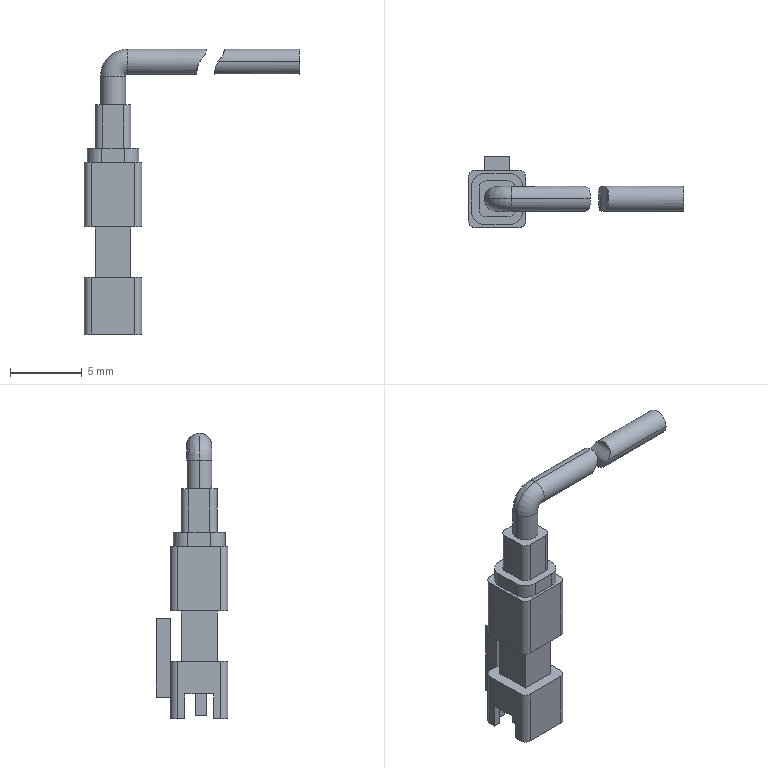Part | STEP file | ASND-0110-2-core power cable | 2 solids | 85 faces | box 15 x 5 x 19.875 mm | volume 201.3 mm3 | plane 59 | cylinder 22 | spline 3 | torus 1 | commonest cylinder face diameters 1 x12 1.75 x6 2 x4